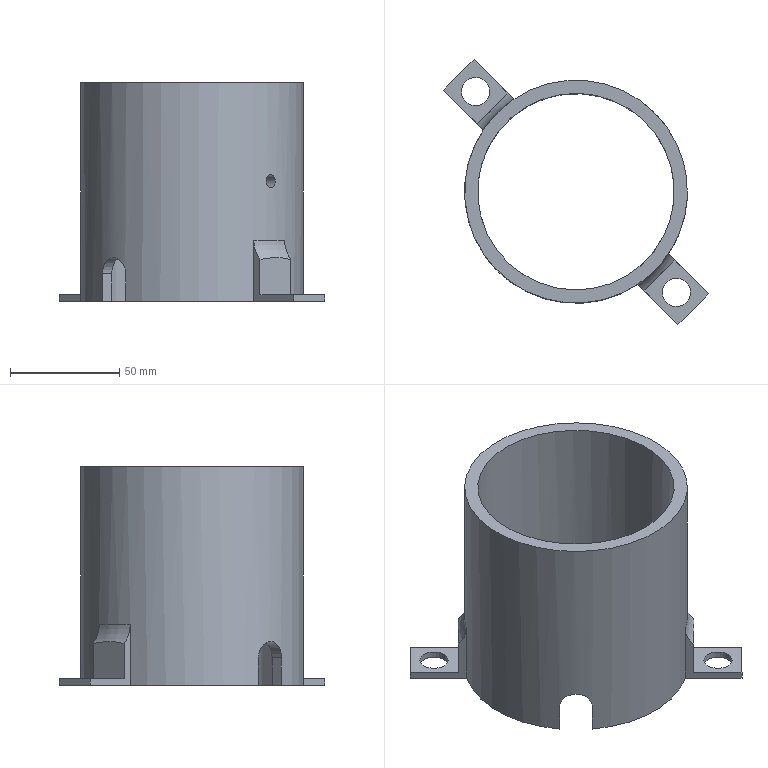Part | NX | features solid 2 | 1 solid | 26 faces | box 121.622 x 121.622 x 100 mm | volume 182276 mm3 | plane 17 | cylinder 7 | torus 2 | commonest cylinder face diameters 13 x2 15 x2 6 x1 90 x1 102 x1
STEP:
#1=CARTESIAN_POINT('',(1436.366,353.634,10.));
#2=VERTEX_POINT('',#1);
#3=CARTESIAN_POINT('',(1440.962,349.038,10.));
#4=DIRECTION('',(0.,0.,-1.));
#5=DIRECTION('',(-0.7071,0.7071,0.));
#6=AXIS2_PLACEMENT_3D('',#3,#4,#5);
#7=CIRCLE('',#6,6.5);
#8=EDGE_CURVE('',#2,#2,#7,.T.);
#9=ORIENTED_EDGE('',*,*,#8,.F.);
#10=EDGE_LOOP('',(#9));
#11=FACE_BOUND('',#10,.T.);
#12=CARTESIAN_POINT('',(1435.974,425.367,10.));
#13=VERTEX_POINT('',#12);
#14=CARTESIAN_POINT('',(1437.433,366.709,10.));
#15=VERTEX_POINT('',#14);
#16=CARTESIAN_POINT('',(1395.,395.,10.));
#17=DIRECTION('',(0.,0.,-1.));
#18=DIRECTION('',(-0.9659,-0.2588,0.));
#19=AXIS2_PLACEMENT_3D('',#16,#17,#18);
#20=CIRCLE('',#19,51.);
#21=EDGE_CURVE('',#13,#15,#20,.T.);
#22=ORIENTED_EDGE('',*,*,#21,.T.);
#23=CARTESIAN_POINT('',(1455.811,348.331,10.));
#24=VERTEX_POINT('',#23);
#25=CARTESIAN_POINT('',(1440.255,363.887,10.));
#26=DIRECTION('',(0.7071,-0.7071,0.));
#27=VECTOR('',#26,1000.);
#28=LINE('',#25,#27);
#29=EDGE_CURVE('',#15,#24,#28,.T.);
#30=ORIENTED_EDGE('',*,*,#29,.T.);
#31=CARTESIAN_POINT('',(1441.669,334.189,10.));
#32=VERTEX_POINT('',#31);
#33=CARTESIAN_POINT('',(1441.669,334.189,10.));
#34=DIRECTION('',(0.7071,0.7071,0.));
#35=VECTOR('',#34,1000.);
#36=LINE('',#33,#35);
#37=EDGE_CURVE('',#32,#24,#36,.T.);
#38=ORIENTED_EDGE('',*,*,#37,.F.);
#39=CARTESIAN_POINT('',(1423.291,352.567,10.));
#40=VERTEX_POINT('',#39);
#41=CARTESIAN_POINT('',(1432.477,343.381,10.));
#42=DIRECTION('',(-0.7071,0.7071,0.));
#43=VECTOR('',#42,1000.);
#44=LINE('',#41,#43);
#45=EDGE_CURVE('',#32,#40,#44,.T.);
#46=ORIENTED_EDGE('',*,*,#45,.T.);
#47=CARTESIAN_POINT('',(1364.633,354.026,10.));
#48=VERTEX_POINT('',#47);
#49=CARTESIAN_POINT('',(1395.,395.,10.));
#50=DIRECTION('',(0.,0.,-1.));
#51=DIRECTION('',(-0.9659,-0.2588,0.));
#52=AXIS2_PLACEMENT_3D('',#49,#50,#51);
#53=CIRCLE('',#52,51.);
#54=EDGE_CURVE('',#40,#48,#53,.T.);
#55=ORIENTED_EDGE('',*,*,#54,.T.);
#56=CARTESIAN_POINT('',(1368.929,358.322,10.));
#57=VERTEX_POINT('',#56);
#58=CARTESIAN_POINT('',(1400.303,389.697,10.));
#59=DIRECTION('',(-0.7071,-0.7071,0.));
#60=VECTOR('',#59,1000.);
#61=LINE('',#58,#60);
#62=EDGE_CURVE('',#57,#48,#61,.T.);
#63=ORIENTED_EDGE('',*,*,#62,.F.);
#64=CARTESIAN_POINT('',(1431.678,421.071,10.));
#65=VERTEX_POINT('',#64);
#66=CARTESIAN_POINT('',(1395.,395.,10.));
#67=DIRECTION('',(0.,0.,-1.));
#68=DIRECTION('',(-0.9659,-0.2588,0.));
#69=AXIS2_PLACEMENT_3D('',#66,#67,#68);
#70=CIRCLE('',#69,45.);
#71=EDGE_CURVE('',#65,#57,#70,.T.);
#72=ORIENTED_EDGE('',*,*,#71,.F.);
#73=CARTESIAN_POINT('',(1400.303,389.697,10.));
#74=DIRECTION('',(-0.7071,-0.7071,0.));
#75=VECTOR('',#74,1000.);
#76=LINE('',#73,#75);
#77=EDGE_CURVE('',#13,#65,#76,.T.);
#78=ORIENTED_EDGE('',*,*,#77,.F.);
#79=EDGE_LOOP('',(#22,#30,#38,#46,#55,#63,#72,#78));
#80=FACE_BOUND('',#79,.T.);
#81=CARTESIAN_POINT('',(1395.,395.,10.));
#82=DIRECTION('',(0.,0.,1.));
#83=DIRECTION('',(-0.7071,0.7071,0.));
#84=AXIS2_PLACEMENT_3D('',#81,#82,#83);
#85=PLANE('',#84);
#86=ADVANCED_FACE('',(#11,#80),#85,.F.);
#87=CARTESIAN_POINT('',(1430.87,358.746,62.012));
#88=VERTEX_POINT('',#87);
#89=CARTESIAN_POINT('',(1429.215,357.17,62.873));
#90=CARTESIAN_POINT('',(1430.865,358.71,61.688));
#91=CARTESIAN_POINT('',(1432.545,360.466,62.447));
#92=CARTESIAN_POINT('',(1433.326,361.356,64.697));
#93=CARTESIAN_POINT('',(1432.83,360.784,67.128));
#94=CARTESIAN_POINT('',(1431.29,359.136,68.311));
#95=CARTESIAN_POINT('',(1429.537,357.457,67.556));
#96=CARTESIAN_POINT('',(1428.644,356.674,65.304));
#97=CARTESIAN_POINT('',(1429.215,357.17,62.873));
#98=CARTESIAN_POINT('',(1430.865,358.71,61.688));
#99=CARTESIAN_POINT('',(1432.545,360.466,62.447));
#100=B_SPLINE_CURVE_WITH_KNOTS('',3,(#89,#90,#91,#92,#93,#94,#95,#96,#97,#98,#99),.UNSPECIFIED.,.T.,.F.,(1,1,1,1,1,1,1,1,1,1,1,1,1,1,1),(-0.007035,-0.00469,-0.002345,0.,0.002345,0.00469,0.007035,0.00938,0.01173,0.01407,0.01642,0.01876,0.02111,0.02345,0.0258),.UNSPECIFIED.);
#101=EDGE_CURVE('',#88,#88,#100,.T.);
#102=ORIENTED_EDGE('',*,*,#101,.F.);
#103=EDGE_LOOP('',(#102));
#104=FACE_BOUND('',#103,.T.);
#105=CARTESIAN_POINT('',(1444.262,408.2,110.));
#106=VERTEX_POINT('',#105);
#107=CARTESIAN_POINT('',(1395.,395.,110.));
#108=DIRECTION('',(0.,0.,-1.));
#109=DIRECTION('',(0.9659,0.2588,0.));
#110=AXIS2_PLACEMENT_3D('',#107,#108,#109);
#111=CIRCLE('',#110,51.);
#112=EDGE_CURVE('',#106,#106,#111,.T.);
#113=ORIENTED_EDGE('',*,*,#112,.T.);
#114=EDGE_LOOP('',(#113));
#115=FACE_BOUND('',#114,.T.);
#116=CARTESIAN_POINT('',(1425.367,435.974,22.5));
#117=VERTEX_POINT('',#116);
#118=CARTESIAN_POINT('',(1435.974,425.367,22.5));
#119=VERTEX_POINT('',#118);
#120=CARTESIAN_POINT('',(1425.367,435.974,22.5));
#121=CARTESIAN_POINT('',(1425.367,435.974,24.46));
#122=CARTESIAN_POINT('',(1426.705,435.029,28.37));
#123=CARTESIAN_POINT('',(1431.168,431.152,30.816));
#124=CARTESIAN_POINT('',(1435.022,426.713,28.365));
#125=CARTESIAN_POINT('',(1435.974,425.367,24.48));
#126=CARTESIAN_POINT('',(1435.974,425.367,22.5));
#127=B_SPLINE_CURVE_WITH_KNOTS('',3,(#120,#121,#122,#123,#124,#125,#126),.UNSPECIFIED.,.F.,.F.,(4,1,1,1,4),(0.03594,0.04181,0.04768,0.05355,0.05942),.UNSPECIFIED.);
#128=EDGE_CURVE('',#117,#119,#127,.T.);
#129=ORIENTED_EDGE('',*,*,#128,.F.);
#130=CARTESIAN_POINT('',(1425.367,435.974,10.));
#131=VERTEX_POINT('',#130);
#132=CARTESIAN_POINT('',(1425.367,435.974,120.));
#133=DIRECTION('',(0.,0.,-1.));
#134=VECTOR('',#133,1000.);
#135=LINE('',#132,#134);
#136=EDGE_CURVE('',#131,#117,#135,.F.);
#137=ORIENTED_EDGE('',*,*,#136,.F.);
#138=CARTESIAN_POINT('',(1366.709,437.433,10.));
#139=VERTEX_POINT('',#138);
#140=CARTESIAN_POINT('',(1395.,395.,10.));
#141=DIRECTION('',(0.,0.,-1.));
#142=DIRECTION('',(-0.9659,-0.2588,0.));
#143=AXIS2_PLACEMENT_3D('',#140,#141,#142);
#144=CIRCLE('',#143,51.);
#145=EDGE_CURVE('',#139,#131,#144,.T.);
#146=ORIENTED_EDGE('',*,*,#145,.F.);
#147=CARTESIAN_POINT('',(1366.709,437.433,38.));
#148=VERTEX_POINT('',#147);
#149=CARTESIAN_POINT('',(1366.709,437.433,10.));
#150=DIRECTION('',(0.,0.,-1.));
#151=VECTOR('',#150,1000.);
#152=LINE('',#149,#151);
#153=EDGE_CURVE('',#139,#148,#152,.F.);
#154=ORIENTED_EDGE('',*,*,#153,.T.);
#155=CARTESIAN_POINT('',(1352.567,423.291,38.));
#156=VERTEX_POINT('',#155);
#157=CARTESIAN_POINT('',(1395.,395.,38.));
#158=DIRECTION('',(0.,0.,1.));
#159=DIRECTION('',(0.9659,0.2588,0.));
#160=AXIS2_PLACEMENT_3D('',#157,#158,#159);
#161=CIRCLE('',#160,51.);
#162=EDGE_CURVE('',#156,#148,#161,.F.);
#163=ORIENTED_EDGE('',*,*,#162,.F.);
#164=CARTESIAN_POINT('',(1352.567,423.291,10.));
#165=VERTEX_POINT('',#164);
#166=CARTESIAN_POINT('',(1352.567,423.291,120.));
#167=DIRECTION('',(0.,0.,-1.));
#168=VECTOR('',#167,1000.);
#169=LINE('',#166,#168);
#170=EDGE_CURVE('',#156,#165,#169,.T.);
#171=ORIENTED_EDGE('',*,*,#170,.T.);
#172=CARTESIAN_POINT('',(1354.026,364.633,10.));
#173=VERTEX_POINT('',#172);
#174=CARTESIAN_POINT('',(1395.,395.,10.));
#175=DIRECTION('',(0.,0.,-1.));
#176=DIRECTION('',(-0.9659,-0.2588,0.));
#177=AXIS2_PLACEMENT_3D('',#174,#175,#176);
#178=CIRCLE('',#177,51.);
#179=EDGE_CURVE('',#173,#165,#178,.T.);
#180=ORIENTED_EDGE('',*,*,#179,.F.);
#181=CARTESIAN_POINT('',(1354.026,364.633,22.5));
#182=VERTEX_POINT('',#181);
#183=CARTESIAN_POINT('',(1354.026,364.633,120.));
#184=DIRECTION('',(0.,0.,-1.));
#185=VECTOR('',#184,1000.);
#186=LINE('',#183,#185);
#187=EDGE_CURVE('',#182,#173,#186,.T.);
#188=ORIENTED_EDGE('',*,*,#187,.F.);
#189=CARTESIAN_POINT('',(1364.633,354.026,22.5));
#190=VERTEX_POINT('',#189);
#191=CARTESIAN_POINT('',(1364.633,354.026,22.5));
#192=CARTESIAN_POINT('',(1364.633,354.026,24.483));
#193=CARTESIAN_POINT('',(1363.29,354.975,28.366));
#194=CARTESIAN_POINT('',(1358.835,358.845,30.816));
#195=CARTESIAN_POINT('',(1354.974,363.292,28.369));
#196=CARTESIAN_POINT('',(1354.026,364.633,24.459));
#197=CARTESIAN_POINT('',(1354.026,364.633,22.5));
#198=B_SPLINE_CURVE_WITH_KNOTS('',3,(#191,#192,#193,#194,#195,#196,#197),.UNSPECIFIED.,.F.,.F.,(4,1,1,1,4),(0.03522,0.04109,0.04696,0.05283,0.0587),.UNSPECIFIED.);
#199=EDGE_CURVE('',#190,#182,#198,.T.);
#200=ORIENTED_EDGE('',*,*,#199,.F.);
#201=CARTESIAN_POINT('',(1364.633,354.026,120.));
#202=DIRECTION('',(0.,0.,-1.));
#203=VECTOR('',#202,1000.);
#204=LINE('',#201,#203);
#205=EDGE_CURVE('',#48,#190,#204,.F.);
#206=ORIENTED_EDGE('',*,*,#205,.F.);
#207=ORIENTED_EDGE('',*,*,#54,.F.);
#208=CARTESIAN_POINT('',(1423.291,352.567,38.));
#209=VERTEX_POINT('',#208);
#210=CARTESIAN_POINT('',(1423.291,352.567,10.));
#211=DIRECTION('',(0.,0.,-1.));
#212=VECTOR('',#211,1000.);
#213=LINE('',#210,#212);
#214=EDGE_CURVE('',#40,#209,#213,.F.);
#215=ORIENTED_EDGE('',*,*,#214,.T.);
#216=CARTESIAN_POINT('',(1437.433,366.709,38.));
#217=VERTEX_POINT('',#216);
#218=CARTESIAN_POINT('',(1395.,395.,38.));
#219=DIRECTION('',(0.,0.,1.));
#220=DIRECTION('',(0.9659,0.2588,0.));
#221=AXIS2_PLACEMENT_3D('',#218,#219,#220);
#222=CIRCLE('',#221,51.);
#223=EDGE_CURVE('',#217,#209,#222,.F.);
#224=ORIENTED_EDGE('',*,*,#223,.F.);
#225=CARTESIAN_POINT('',(1437.433,366.709,120.));
#226=DIRECTION('',(0.,0.,-1.));
#227=VECTOR('',#226,1000.);
#228=LINE('',#225,#227);
#229=EDGE_CURVE('',#217,#15,#228,.T.);
#230=ORIENTED_EDGE('',*,*,#229,.T.);
#231=ORIENTED_EDGE('',*,*,#21,.F.);
#232=CARTESIAN_POINT('',(1435.974,425.367,120.));
#233=DIRECTION('',(0.,0.,-1.));
#234=VECTOR('',#233,1000.);
#235=LINE('',#232,#234);
#236=EDGE_CURVE('',#119,#13,#235,.T.);
#237=ORIENTED_EDGE('',*,*,#236,.F.);
#238=EDGE_LOOP('',(#129,#137,#146,#154,#163,#171,#180,#188,#200,#206,#207,#215,#224,#230,#231,#237));
#239=FACE_BOUND('',#238,.T.);
#240=CARTESIAN_POINT('',(1395.,395.,120.));
#241=DIRECTION('',(0.,0.,-1.));
#242=DIRECTION('',(0.7071,-0.7071,0.));
#243=AXIS2_PLACEMENT_3D('',#240,#241,#242);
#244=CYLINDRICAL_SURFACE('',#243,51.);
#245=ADVANCED_FACE('',(#104,#115,#239),#244,.T.);
#246=CARTESIAN_POINT('',(1431.678,421.071,22.5));
#247=VERTEX_POINT('',#246);
#248=CARTESIAN_POINT('',(1431.678,421.071,120.));
#249=DIRECTION('',(0.,0.,-1.));
#250=VECTOR('',#249,1000.);
#251=LINE('',#248,#250);
#252=EDGE_CURVE('',#247,#65,#251,.T.);
#253=ORIENTED_EDGE('',*,*,#252,.T.);
#254=ORIENTED_EDGE('',*,*,#71,.T.);
#255=CARTESIAN_POINT('',(1368.929,358.322,22.5));
#256=VERTEX_POINT('',#255);
#257=CARTESIAN_POINT('',(1368.929,358.322,120.));
#258=DIRECTION('',(0.,0.,-1.));
#259=VECTOR('',#258,1000.);
#260=LINE('',#257,#259);
#261=EDGE_CURVE('',#57,#256,#260,.F.);
#262=ORIENTED_EDGE('',*,*,#261,.T.);
#263=CARTESIAN_POINT('',(1358.322,368.929,22.5));
#264=VERTEX_POINT('',#263);
#265=CARTESIAN_POINT('',(1368.929,358.322,22.5));
#266=CARTESIAN_POINT('',(1368.929,358.322,24.482));
#267=CARTESIAN_POINT('',(1367.559,359.244,28.366));
#268=CARTESIAN_POINT('',(1363.064,363.075,30.817));
#269=CARTESIAN_POINT('',(1359.243,367.561,28.368));
#270=CARTESIAN_POINT('',(1358.322,368.929,24.46));
#271=CARTESIAN_POINT('',(1358.322,368.929,22.5));
#272=B_SPLINE_CURVE_WITH_KNOTS('',3,(#265,#266,#267,#268,#269,#270,#271),.UNSPECIFIED.,.F.,.F.,(4,1,1,1,4),(0.03524,0.04111,0.04698,0.05285,0.05872),.UNSPECIFIED.);
#273=EDGE_CURVE('',#256,#264,#272,.T.);
#274=ORIENTED_EDGE('',*,*,#273,.T.);
#275=CARTESIAN_POINT('',(1358.322,368.929,10.));
#276=VERTEX_POINT('',#275);
#277=CARTESIAN_POINT('',(1358.322,368.929,120.));
#278=DIRECTION('',(0.,0.,-1.));
#279=VECTOR('',#278,1000.);
#280=LINE('',#277,#279);
#281=EDGE_CURVE('',#264,#276,#280,.T.);
#282=ORIENTED_EDGE('',*,*,#281,.T.);
#283=CARTESIAN_POINT('',(1421.071,431.678,10.));
#284=VERTEX_POINT('',#283);
#285=CARTESIAN_POINT('',(1395.,395.,10.));
#286=DIRECTION('',(0.,0.,-1.));
#287=DIRECTION('',(-0.9659,-0.2588,0.));
#288=AXIS2_PLACEMENT_3D('',#285,#286,#287);
#289=CIRCLE('',#288,45.);
#290=EDGE_CURVE('',#276,#284,#289,.T.);
#291=ORIENTED_EDGE('',*,*,#290,.T.);
#292=CARTESIAN_POINT('',(1421.071,431.678,22.5));
#293=VERTEX_POINT('',#292);
#294=CARTESIAN_POINT('',(1421.071,431.678,120.));
#295=DIRECTION('',(0.,0.,-1.));
#296=VECTOR('',#295,1000.);
#297=LINE('',#294,#296);
#298=EDGE_CURVE('',#284,#293,#297,.F.);
#299=ORIENTED_EDGE('',*,*,#298,.T.);
#300=CARTESIAN_POINT('',(1421.071,431.678,22.5));
#301=CARTESIAN_POINT('',(1421.071,431.678,24.485));
#302=CARTESIAN_POINT('',(1422.445,430.753,28.364));
#303=CARTESIAN_POINT('',(1426.924,426.936,30.816));
#304=CARTESIAN_POINT('',(1430.753,422.446,28.37));
#305=CARTESIAN_POINT('',(1431.678,421.071,24.485));
#306=CARTESIAN_POINT('',(1431.678,421.071,22.5));
#307=B_SPLINE_CURVE_WITH_KNOTS('',3,(#300,#301,#302,#303,#304,#305,#306),.UNSPECIFIED.,.F.,.F.,(4,1,1,1,4),(0.,0.005871,0.01174,0.01761,0.02348),.UNSPECIFIED.);
#308=EDGE_CURVE('',#293,#247,#307,.T.);
#309=ORIENTED_EDGE('',*,*,#308,.T.);
#310=EDGE_LOOP('',(#253,#254,#262,#274,#282,#291,#299,#309));
#311=FACE_BOUND('',#310,.T.);
#312=CARTESIAN_POINT('',(1426.631,362.992,62.012));
#313=VERTEX_POINT('',#312);
#314=CARTESIAN_POINT('',(1424.97,361.42,62.869));
#315=CARTESIAN_POINT('',(1426.628,362.955,61.688));
#316=CARTESIAN_POINT('',(1428.302,364.714,62.451));
#317=CARTESIAN_POINT('',(1429.073,365.609,64.702));
#318=CARTESIAN_POINT('',(1428.579,365.029,67.132));
#319=CARTESIAN_POINT('',(1427.046,363.373,68.311));
#320=CARTESIAN_POINT('',(1425.288,361.7,67.552));
#321=CARTESIAN_POINT('',(1424.391,360.926,65.299));
#322=CARTESIAN_POINT('',(1424.97,361.42,62.869));
#323=CARTESIAN_POINT('',(1426.628,362.955,61.688));
#324=CARTESIAN_POINT('',(1428.302,364.714,62.451));
#325=B_SPLINE_CURVE_WITH_KNOTS('',3,(#314,#315,#316,#317,#318,#319,#320,#321,#322,#323,#324),.UNSPECIFIED.,.T.,.F.,(1,1,1,1,1,1,1,1,1,1,1,1,1,1,1),(-0.007036,-0.00469,-0.002345,0.,0.002345,0.00469,0.007036,0.009381,0.01173,0.01407,0.01642,0.01876,0.02111,0.02345,0.0258),.UNSPECIFIED.);
#326=EDGE_CURVE('',#313,#313,#325,.T.);
#327=ORIENTED_EDGE('',*,*,#326,.T.);
#328=EDGE_LOOP('',(#327));
#329=FACE_BOUND('',#328,.T.);
#330=CARTESIAN_POINT('',(1438.467,406.647,110.));
#331=VERTEX_POINT('',#330);
#332=CARTESIAN_POINT('',(1395.,395.,110.));
#333=DIRECTION('',(0.,0.,-1.));
#334=DIRECTION('',(0.9659,0.2588,0.));
#335=AXIS2_PLACEMENT_3D('',#332,#333,#334);
#336=CIRCLE('',#335,45.);
#337=EDGE_CURVE('',#331,#331,#336,.T.);
#338=ORIENTED_EDGE('',*,*,#337,.F.);
#339=EDGE_LOOP('',(#338));
#340=FACE_BOUND('',#339,.T.);
#341=CARTESIAN_POINT('',(1395.,395.,120.));
#342=DIRECTION('',(0.,0.,-1.));
#343=DIRECTION('',(0.7071,-0.7071,0.));
#344=AXIS2_PLACEMENT_3D('',#341,#342,#343);
#345=CYLINDRICAL_SURFACE('',#344,45.);
#346=ADVANCED_FACE('',(#311,#329,#340),#345,.F.);
#347=ORIENTED_EDGE('',*,*,#337,.T.);
#348=EDGE_LOOP('',(#347));
#349=FACE_BOUND('',#348,.T.);
#350=ORIENTED_EDGE('',*,*,#112,.F.);
#351=EDGE_LOOP('',(#350));
#352=FACE_BOUND('',#351,.T.);
#353=CARTESIAN_POINT('',(1395.,395.,110.));
#354=DIRECTION('',(0.,0.,1.));
#355=DIRECTION('',(-0.7071,0.7071,0.));
#356=AXIS2_PLACEMENT_3D('',#353,#354,#355);
#357=PLANE('',#356);
#358=ADVANCED_FACE('',(#349,#352),#357,.T.);
#359=ORIENTED_EDGE('',*,*,#290,.F.);
#360=CARTESIAN_POINT('',(1389.697,400.303,10.));
#361=DIRECTION('',(0.7071,0.7071,0.));
#362=VECTOR('',#361,1000.);
#363=LINE('',#360,#362);
#364=EDGE_CURVE('',#173,#276,#363,.T.);
#365=ORIENTED_EDGE('',*,*,#364,.F.);
#366=ORIENTED_EDGE('',*,*,#179,.T.);
#367=CARTESIAN_POINT('',(1334.189,441.669,10.));
#368=VERTEX_POINT('',#367);
#369=CARTESIAN_POINT('',(1349.745,426.113,10.));
#370=DIRECTION('',(-0.7071,0.7071,0.));
#371=VECTOR('',#370,1000.);
#372=LINE('',#369,#371);
#373=EDGE_CURVE('',#165,#368,#372,.T.);
#374=ORIENTED_EDGE('',*,*,#373,.T.);
#375=CARTESIAN_POINT('',(1348.331,455.811,10.));
#376=VERTEX_POINT('',#375);
#377=CARTESIAN_POINT('',(1348.331,455.811,10.));
#378=DIRECTION('',(-0.7071,-0.7071,0.));
#379=VECTOR('',#378,1000.);
#380=LINE('',#377,#379);
#381=EDGE_CURVE('',#376,#368,#380,.T.);
#382=ORIENTED_EDGE('',*,*,#381,.F.);
#383=CARTESIAN_POINT('',(1357.523,446.619,10.));
#384=DIRECTION('',(0.7071,-0.7071,0.));
#385=VECTOR('',#384,1000.);
#386=LINE('',#383,#385);
#387=EDGE_CURVE('',#376,#139,#386,.T.);
#388=ORIENTED_EDGE('',*,*,#387,.T.);
#389=ORIENTED_EDGE('',*,*,#145,.T.);
#390=CARTESIAN_POINT('',(1389.697,400.303,10.));
#391=DIRECTION('',(0.7071,0.7071,0.));
#392=VECTOR('',#391,1000.);
#393=LINE('',#390,#392);
#394=EDGE_CURVE('',#284,#131,#393,.T.);
#395=ORIENTED_EDGE('',*,*,#394,.F.);
#396=EDGE_LOOP('',(#359,#365,#366,#374,#382,#388,#389,#395));
#397=FACE_BOUND('',#396,.T.);
#398=CARTESIAN_POINT('',(1344.442,445.558,10.));
#399=VERTEX_POINT('',#398);
#400=CARTESIAN_POINT('',(1349.038,440.962,10.));
#401=DIRECTION('',(0.,0.,-1.));
#402=DIRECTION('',(-0.7071,0.7071,0.));
#403=AXIS2_PLACEMENT_3D('',#400,#401,#402);
#404=CIRCLE('',#403,6.5);
#405=EDGE_CURVE('',#399,#399,#404,.T.);
#406=ORIENTED_EDGE('',*,*,#405,.F.);
#407=EDGE_LOOP('',(#406));
#408=FACE_BOUND('',#407,.T.);
#409=CARTESIAN_POINT('',(1395.,395.,10.));
#410=DIRECTION('',(0.,0.,1.));
#411=DIRECTION('',(-0.7071,0.7071,0.));
#412=AXIS2_PLACEMENT_3D('',#409,#410,#411);
#413=PLANE('',#412);
#414=ADVANCED_FACE('',(#397,#408),#413,.F.);
#415=ORIENTED_EDGE('',*,*,#45,.F.);
#416=CARTESIAN_POINT('',(1441.669,334.189,13.));
#417=VERTEX_POINT('',#416);
#418=CARTESIAN_POINT('',(1441.669,334.189,13.));
#419=DIRECTION('',(0.,0.,-1.));
#420=VECTOR('',#419,1000.);
#421=LINE('',#418,#420);
#422=EDGE_CURVE('',#417,#32,#421,.T.);
#423=ORIENTED_EDGE('',*,*,#422,.F.);
#424=CARTESIAN_POINT('',(1426.113,349.745,13.));
#425=VERTEX_POINT('',#424);
#426=CARTESIAN_POINT('',(1432.477,343.381,13.));
#427=DIRECTION('',(0.7071,-0.7071,0.));
#428=VECTOR('',#427,1000.);
#429=LINE('',#426,#428);
#430=EDGE_CURVE('',#425,#417,#429,.T.);
#431=ORIENTED_EDGE('',*,*,#430,.F.);
#432=CARTESIAN_POINT('',(1426.113,349.745,29.13));
#433=VERTEX_POINT('',#432);
#434=CARTESIAN_POINT('',(1426.113,349.745,35.));
#435=DIRECTION('',(0.,0.,-1.));
#436=VECTOR('',#435,1000.);
#437=LINE('',#434,#436);
#438=EDGE_CURVE('',#433,#425,#437,.T.);
#439=ORIENTED_EDGE('',*,*,#438,.F.);
#440=CARTESIAN_POINT('',(1423.291,352.567,38.));
#441=CARTESIAN_POINT('',(1423.291,352.567,34.628));
#442=CARTESIAN_POINT('',(1424.362,351.496,31.348));
#443=CARTESIAN_POINT('',(1426.113,349.745,29.13));
#444=B_SPLINE_CURVE_WITH_KNOTS('',3,(#440,#441,#442,#443),.UNSPECIFIED.,.F.,.F.,(4,4),(0.,0.00997),.UNSPECIFIED.);
#445=EDGE_CURVE('',#209,#433,#444,.T.);
#446=ORIENTED_EDGE('',*,*,#445,.F.);
#447=ORIENTED_EDGE('',*,*,#214,.F.);
#448=EDGE_LOOP('',(#415,#423,#431,#439,#446,#447));
#449=FACE_BOUND('',#448,.T.);
#450=CARTESIAN_POINT('',(1432.477,343.381,35.));
#451=DIRECTION('',(0.7071,0.7071,0.));
#452=DIRECTION('',(0.7071,-0.7071,0.));
#453=AXIS2_PLACEMENT_3D('',#450,#451,#452);
#454=PLANE('',#453);
#455=ADVANCED_FACE('',(#449),#454,.F.);
#456=CARTESIAN_POINT('',(1440.255,363.887,29.13));
#457=VERTEX_POINT('',#456);
#458=CARTESIAN_POINT('',(1440.255,363.887,13.));
#459=VERTEX_POINT('',#458);
#460=CARTESIAN_POINT('',(1440.255,363.887,35.));
#461=DIRECTION('',(0.,0.,-1.));
#462=VECTOR('',#461,1000.);
#463=LINE('',#460,#462);
#464=EDGE_CURVE('',#457,#459,#463,.T.);
#465=ORIENTED_EDGE('',*,*,#464,.T.);
#466=CARTESIAN_POINT('',(1455.811,348.331,13.));
#467=VERTEX_POINT('',#466);
#468=CARTESIAN_POINT('',(1462.175,341.967,13.));
#469=DIRECTION('',(-0.7071,0.7071,0.));
#470=VECTOR('',#469,1000.);
#471=LINE('',#468,#470);
#472=EDGE_CURVE('',#467,#459,#471,.T.);
#473=ORIENTED_EDGE('',*,*,#472,.F.);
#474=CARTESIAN_POINT('',(1455.811,348.331,13.));
#475=DIRECTION('',(0.,0.,-1.));
#476=VECTOR('',#475,1000.);
#477=LINE('',#474,#476);
#478=EDGE_CURVE('',#467,#24,#477,.T.);
#479=ORIENTED_EDGE('',*,*,#478,.T.);
#480=ORIENTED_EDGE('',*,*,#29,.F.);
#481=ORIENTED_EDGE('',*,*,#229,.F.);
#482=CARTESIAN_POINT('',(1440.255,363.887,29.13));
#483=CARTESIAN_POINT('',(1438.495,365.647,31.359));
#484=CARTESIAN_POINT('',(1437.433,366.709,34.631));
#485=CARTESIAN_POINT('',(1437.433,366.709,38.));
#486=B_SPLINE_CURVE_WITH_KNOTS('',3,(#482,#483,#484,#485),.UNSPECIFIED.,.F.,.F.,(4,4),(0.00893,0.01889),.UNSPECIFIED.);
#487=EDGE_CURVE('',#457,#217,#486,.T.);
#488=ORIENTED_EDGE('',*,*,#487,.F.);
#489=EDGE_LOOP('',(#465,#473,#479,#480,#481,#488));
#490=FACE_BOUND('',#489,.T.);
#491=CARTESIAN_POINT('',(1440.255,363.887,35.));
#492=DIRECTION('',(-0.7071,-0.7071,0.));
#493=DIRECTION('',(-0.7071,0.7071,0.));
#494=AXIS2_PLACEMENT_3D('',#491,#492,#493);
#495=PLANE('',#494);
#496=ADVANCED_FACE('',(#490),#495,.F.);
#497=ORIENTED_EDGE('',*,*,#464,.F.);
#498=CARTESIAN_POINT('',(1426.113,349.745,29.13));
#499=CARTESIAN_POINT('',(1428.44,352.072,29.676));
#500=CARTESIAN_POINT('',(1431.947,355.58,30.244));
#501=CARTESIAN_POINT('',(1436.083,359.715,29.934));
#502=CARTESIAN_POINT('',(1438.173,361.805,29.579));
#503=CARTESIAN_POINT('',(1439.351,362.984,29.337));
#504=CARTESIAN_POINT('',(1439.976,363.608,29.195));
#505=CARTESIAN_POINT('',(1440.255,363.887,29.13));
#506=B_SPLINE_CURVE_WITH_KNOTS('',3,(#498,#499,#500,#501,#502,#503,#504,#505),.UNSPECIFIED.,.F.,.F.,(4,1,1,1,1,4),(0.2077,0.2173,0.2221,0.2245,0.2257,0.2269),.UNSPECIFIED.);
#507=EDGE_CURVE('',#457,#433,#506,.F.);
#508=ORIENTED_EDGE('',*,*,#507,.T.);
#509=ORIENTED_EDGE('',*,*,#438,.T.);
#510=CARTESIAN_POINT('',(1440.255,363.887,13.));
#511=DIRECTION('',(-0.7071,-0.7071,0.));
#512=VECTOR('',#511,1000.);
#513=LINE('',#510,#512);
#514=EDGE_CURVE('',#459,#425,#513,.T.);
#515=ORIENTED_EDGE('',*,*,#514,.F.);
#516=EDGE_LOOP('',(#497,#508,#509,#515));
#517=FACE_BOUND('',#516,.T.);
#518=CARTESIAN_POINT('',(1440.255,363.887,35.));
#519=DIRECTION('',(-0.7071,0.7071,0.));
#520=DIRECTION('',(0.,0.,-1.));
#521=AXIS2_PLACEMENT_3D('',#518,#519,#520);
#522=PLANE('',#521);
#523=ADVANCED_FACE('',(#517),#522,.F.);
#524=ORIENTED_EDGE('',*,*,#387,.F.);
#525=CARTESIAN_POINT('',(1348.331,455.811,13.));
#526=VERTEX_POINT('',#525);
#527=CARTESIAN_POINT('',(1348.331,455.811,13.));
#528=DIRECTION('',(0.,0.,-1.));
#529=VECTOR('',#528,1000.);
#530=LINE('',#527,#529);
#531=EDGE_CURVE('',#526,#376,#530,.T.);
#532=ORIENTED_EDGE('',*,*,#531,.F.);
#533=CARTESIAN_POINT('',(1363.887,440.255,13.));
#534=VERTEX_POINT('',#533);
#535=CARTESIAN_POINT('',(1357.523,446.619,13.));
#536=DIRECTION('',(-0.7071,0.7071,0.));
#537=VECTOR('',#536,1000.);
#538=LINE('',#535,#537);
#539=EDGE_CURVE('',#534,#526,#538,.T.);
#540=ORIENTED_EDGE('',*,*,#539,.F.);
#541=CARTESIAN_POINT('',(1363.887,440.255,29.13));
#542=VERTEX_POINT('',#541);
#543=CARTESIAN_POINT('',(1363.887,440.255,35.));
#544=DIRECTION('',(0.,0.,-1.));
#545=VECTOR('',#544,1000.);
#546=LINE('',#543,#545);
#547=EDGE_CURVE('',#542,#534,#546,.T.);
#548=ORIENTED_EDGE('',*,*,#547,.F.);
#549=CARTESIAN_POINT('',(1366.709,437.433,38.));
#550=CARTESIAN_POINT('',(1366.709,437.433,34.628));
#551=CARTESIAN_POINT('',(1365.638,438.504,31.348));
#552=CARTESIAN_POINT('',(1363.887,440.255,29.13));
#553=B_SPLINE_CURVE_WITH_KNOTS('',3,(#549,#550,#551,#552),.UNSPECIFIED.,.F.,.F.,(4,4),(0.,0.00997),.UNSPECIFIED.);
#554=EDGE_CURVE('',#148,#542,#553,.T.);
#555=ORIENTED_EDGE('',*,*,#554,.F.);
#556=ORIENTED_EDGE('',*,*,#153,.F.);
#557=EDGE_LOOP('',(#524,#532,#540,#548,#555,#556));
#558=FACE_BOUND('',#557,.T.);
#559=CARTESIAN_POINT('',(1357.523,446.619,35.));
#560=DIRECTION('',(-0.7071,-0.7071,0.));
#561=DIRECTION('',(-0.7071,0.7071,0.));
#562=AXIS2_PLACEMENT_3D('',#559,#560,#561);
#563=PLANE('',#562);
#564=ADVANCED_FACE('',(#558),#563,.F.);
#565=CARTESIAN_POINT('',(1349.745,426.113,29.13));
#566=VERTEX_POINT('',#565);
#567=CARTESIAN_POINT('',(1349.745,426.113,13.));
#568=VERTEX_POINT('',#567);
#569=CARTESIAN_POINT('',(1349.745,426.113,35.));
#570=DIRECTION('',(0.,0.,-1.));
#571=VECTOR('',#570,1000.);
#572=LINE('',#569,#571);
#573=EDGE_CURVE('',#566,#568,#572,.T.);
#574=ORIENTED_EDGE('',*,*,#573,.T.);
#575=CARTESIAN_POINT('',(1334.189,441.669,13.));
#576=VERTEX_POINT('',#575);
#577=CARTESIAN_POINT('',(1327.825,448.033,13.));
#578=DIRECTION('',(0.7071,-0.7071,0.));
#579=VECTOR('',#578,1000.);
#580=LINE('',#577,#579);
#581=EDGE_CURVE('',#576,#568,#580,.T.);
#582=ORIENTED_EDGE('',*,*,#581,.F.);
#583=CARTESIAN_POINT('',(1334.189,441.669,13.));
#584=DIRECTION('',(0.,0.,-1.));
#585=VECTOR('',#584,1000.);
#586=LINE('',#583,#585);
#587=EDGE_CURVE('',#576,#368,#586,.T.);
#588=ORIENTED_EDGE('',*,*,#587,.T.);
#589=ORIENTED_EDGE('',*,*,#373,.F.);
#590=ORIENTED_EDGE('',*,*,#170,.F.);
#591=CARTESIAN_POINT('',(1349.745,426.113,29.13));
#592=CARTESIAN_POINT('',(1351.505,424.353,31.359));
#593=CARTESIAN_POINT('',(1352.567,423.291,34.631));
#594=CARTESIAN_POINT('',(1352.567,423.291,38.));
#595=B_SPLINE_CURVE_WITH_KNOTS('',3,(#591,#592,#593,#594),.UNSPECIFIED.,.F.,.F.,(4,4),(0.00893,0.01889),.UNSPECIFIED.);
#596=EDGE_CURVE('',#566,#156,#595,.T.);
#597=ORIENTED_EDGE('',*,*,#596,.F.);
#598=EDGE_LOOP('',(#574,#582,#588,#589,#590,#597));
#599=FACE_BOUND('',#598,.T.);
#600=CARTESIAN_POINT('',(1349.745,426.113,35.));
#601=DIRECTION('',(0.7071,0.7071,0.));
#602=DIRECTION('',(0.,0.,1.));
#603=AXIS2_PLACEMENT_3D('',#600,#601,#602);
#604=PLANE('',#603);
#605=ADVANCED_FACE('',(#599),#604,.F.);
#606=ORIENTED_EDGE('',*,*,#573,.F.);
#607=CARTESIAN_POINT('',(1363.887,440.255,29.13));
#608=CARTESIAN_POINT('',(1361.56,437.928,29.676));
#609=CARTESIAN_POINT('',(1358.053,434.42,30.244));
#610=CARTESIAN_POINT('',(1353.917,430.285,29.934));
#611=CARTESIAN_POINT('',(1351.827,428.195,29.579));
#612=CARTESIAN_POINT('',(1350.649,427.016,29.337));
#613=CARTESIAN_POINT('',(1350.024,426.392,29.195));
#614=CARTESIAN_POINT('',(1349.745,426.113,29.13));
#615=B_SPLINE_CURVE_WITH_KNOTS('',3,(#607,#608,#609,#610,#611,#612,#613,#614),.UNSPECIFIED.,.F.,.F.,(4,1,1,1,1,4),(0.2077,0.2173,0.2221,0.2245,0.2257,0.2269),.UNSPECIFIED.);
#616=EDGE_CURVE('',#566,#542,#615,.F.);
#617=ORIENTED_EDGE('',*,*,#616,.T.);
#618=ORIENTED_EDGE('',*,*,#547,.T.);
#619=CARTESIAN_POINT('',(1349.745,426.113,13.));
#620=DIRECTION('',(0.7071,0.7071,0.));
#621=VECTOR('',#620,1000.);
#622=LINE('',#619,#621);
#623=EDGE_CURVE('',#568,#534,#622,.T.);
#624=ORIENTED_EDGE('',*,*,#623,.F.);
#625=EDGE_LOOP('',(#606,#617,#618,#624));
#626=FACE_BOUND('',#625,.T.);
#627=CARTESIAN_POINT('',(1349.745,426.113,35.));
#628=DIRECTION('',(0.7071,-0.7071,0.));
#629=DIRECTION('',(0.,0.,1.));
#630=AXIS2_PLACEMENT_3D('',#627,#628,#629);
#631=PLANE('',#630);
#632=ADVANCED_FACE('',(#626),#631,.F.);
#633=ORIENTED_EDGE('',*,*,#381,.T.);
#634=ORIENTED_EDGE('',*,*,#587,.F.);
#635=CARTESIAN_POINT('',(1348.331,455.811,13.));
#636=DIRECTION('',(-0.7071,-0.7071,0.));
#637=VECTOR('',#636,1000.);
#638=LINE('',#635,#637);
#639=EDGE_CURVE('',#526,#576,#638,.T.);
#640=ORIENTED_EDGE('',*,*,#639,.F.);
#641=ORIENTED_EDGE('',*,*,#531,.T.);
#642=EDGE_LOOP('',(#633,#634,#640,#641));
#643=FACE_BOUND('',#642,.T.);
#644=CARTESIAN_POINT('',(1348.331,455.811,13.));
#645=DIRECTION('',(-0.7071,0.7071,0.));
#646=DIRECTION('',(0.,0.,-1.));
#647=AXIS2_PLACEMENT_3D('',#644,#645,#646);
#648=PLANE('',#647);
#649=ADVANCED_FACE('',(#643),#648,.T.);
#650=CARTESIAN_POINT('',(1344.442,445.558,13.));
#651=VERTEX_POINT('',#650);
#652=CARTESIAN_POINT('',(1349.038,440.962,13.));
#653=DIRECTION('',(0.,0.,-1.));
#654=DIRECTION('',(-0.7071,0.7071,0.));
#655=AXIS2_PLACEMENT_3D('',#652,#653,#654);
#656=CIRCLE('',#655,6.5);
#657=EDGE_CURVE('',#651,#651,#656,.T.);
#658=ORIENTED_EDGE('',*,*,#657,.F.);
#659=EDGE_LOOP('',(#658));
#660=FACE_BOUND('',#659,.T.);
#661=ORIENTED_EDGE('',*,*,#405,.T.);
#662=EDGE_LOOP('',(#661));
#663=FACE_BOUND('',#662,.T.);
#664=CARTESIAN_POINT('',(1349.038,440.962,13.));
#665=DIRECTION('',(0.,0.,-1.));
#666=DIRECTION('',(0.7071,-0.7071,0.));
#667=AXIS2_PLACEMENT_3D('',#664,#665,#666);
#668=CYLINDRICAL_SURFACE('',#667,6.5);
#669=ADVANCED_FACE('',(#660,#663),#668,.F.);
#670=ORIENTED_EDGE('',*,*,#639,.T.);
#671=ORIENTED_EDGE('',*,*,#581,.T.);
#672=ORIENTED_EDGE('',*,*,#623,.T.);
#673=ORIENTED_EDGE('',*,*,#539,.T.);
#674=EDGE_LOOP('',(#670,#671,#672,#673));
#675=FACE_BOUND('',#674,.T.);
#676=ORIENTED_EDGE('',*,*,#657,.T.);
#677=EDGE_LOOP('',(#676));
#678=FACE_BOUND('',#677,.T.);
#679=CARTESIAN_POINT('',(1327.825,448.033,13.));
#680=DIRECTION('',(0.,0.,-1.));
#681=DIRECTION('',(0.7071,-0.7071,0.));
#682=AXIS2_PLACEMENT_3D('',#679,#680,#681);
#683=PLANE('',#682);
#684=ADVANCED_FACE('',(#675,#678),#683,.F.);
#685=ORIENTED_EDGE('',*,*,#37,.T.);
#686=ORIENTED_EDGE('',*,*,#478,.F.);
#687=CARTESIAN_POINT('',(1441.669,334.189,13.));
#688=DIRECTION('',(0.7071,0.7071,0.));
#689=VECTOR('',#688,1000.);
#690=LINE('',#687,#689);
#691=EDGE_CURVE('',#417,#467,#690,.T.);
#692=ORIENTED_EDGE('',*,*,#691,.F.);
#693=ORIENTED_EDGE('',*,*,#422,.T.);
#694=EDGE_LOOP('',(#685,#686,#692,#693));
#695=FACE_BOUND('',#694,.T.);
#696=CARTESIAN_POINT('',(1441.669,334.189,13.));
#697=DIRECTION('',(0.7071,-0.7071,0.));
#698=DIRECTION('',(0.,0.,1.));
#699=AXIS2_PLACEMENT_3D('',#696,#697,#698);
#700=PLANE('',#699);
#701=ADVANCED_FACE('',(#695),#700,.T.);
#702=CARTESIAN_POINT('',(1436.366,353.634,13.));
#703=VERTEX_POINT('',#702);
#704=CARTESIAN_POINT('',(1440.962,349.038,13.));
#705=DIRECTION('',(0.,0.,-1.));
#706=DIRECTION('',(-0.7071,0.7071,0.));
#707=AXIS2_PLACEMENT_3D('',#704,#705,#706);
#708=CIRCLE('',#707,6.5);
#709=EDGE_CURVE('',#703,#703,#708,.T.);
#710=ORIENTED_EDGE('',*,*,#709,.F.);
#711=EDGE_LOOP('',(#710));
#712=FACE_BOUND('',#711,.T.);
#713=ORIENTED_EDGE('',*,*,#8,.T.);
#714=EDGE_LOOP('',(#713));
#715=FACE_BOUND('',#714,.T.);
#716=CARTESIAN_POINT('',(1440.962,349.038,13.));
#717=DIRECTION('',(0.,0.,-1.));
#718=DIRECTION('',(0.7071,-0.7071,0.));
#719=AXIS2_PLACEMENT_3D('',#716,#717,#718);
#720=CYLINDRICAL_SURFACE('',#719,6.5);
#721=ADVANCED_FACE('',(#712,#715),#720,.F.);
#722=ORIENTED_EDGE('',*,*,#691,.T.);
#723=ORIENTED_EDGE('',*,*,#472,.T.);
#724=ORIENTED_EDGE('',*,*,#514,.T.);
#725=ORIENTED_EDGE('',*,*,#430,.T.);
#726=EDGE_LOOP('',(#722,#723,#724,#725));
#727=FACE_BOUND('',#726,.T.);
#728=ORIENTED_EDGE('',*,*,#709,.T.);
#729=EDGE_LOOP('',(#728));
#730=FACE_BOUND('',#729,.T.);
#731=CARTESIAN_POINT('',(1462.175,341.967,13.));
#732=DIRECTION('',(0.,0.,-1.));
#733=DIRECTION('',(0.7071,-0.7071,0.));
#734=AXIS2_PLACEMENT_3D('',#731,#732,#733);
#735=PLANE('',#734);
#736=ADVANCED_FACE('',(#727,#730),#735,.F.);
#737=ORIENTED_EDGE('',*,*,#487,.T.);
#738=ORIENTED_EDGE('',*,*,#223,.T.);
#739=ORIENTED_EDGE('',*,*,#445,.T.);
#740=ORIENTED_EDGE('',*,*,#507,.F.);
#741=EDGE_LOOP('',(#737,#738,#739,#740));
#742=FACE_BOUND('',#741,.T.);
#743=CARTESIAN_POINT('',(1395.,395.,38.));
#744=DIRECTION('',(0.,0.,1.));
#745=DIRECTION('',(-0.7071,0.7071,0.));
#746=AXIS2_PLACEMENT_3D('',#743,#744,#745);
#747=TOROIDAL_SURFACE('',#746,63.,12.);
#748=ADVANCED_FACE('',(#742),#747,.F.);
#749=ORIENTED_EDGE('',*,*,#596,.T.);
#750=ORIENTED_EDGE('',*,*,#162,.T.);
#751=ORIENTED_EDGE('',*,*,#554,.T.);
#752=ORIENTED_EDGE('',*,*,#616,.F.);
#753=EDGE_LOOP('',(#749,#750,#751,#752));
#754=FACE_BOUND('',#753,.T.);
#755=CARTESIAN_POINT('',(1395.,395.,38.));
#756=DIRECTION('',(0.,0.,1.));
#757=DIRECTION('',(-0.7071,0.7071,0.));
#758=AXIS2_PLACEMENT_3D('',#755,#756,#757);
#759=TOROIDAL_SURFACE('',#758,63.,12.);
#760=ADVANCED_FACE('',(#754),#759,.F.);
#761=ORIENTED_EDGE('',*,*,#326,.F.);
#762=EDGE_LOOP('',(#761));
#763=FACE_BOUND('',#762,.T.);
#764=ORIENTED_EDGE('',*,*,#101,.T.);
#765=EDGE_LOOP('',(#764));
#766=FACE_BOUND('',#765,.T.);
#767=CARTESIAN_POINT('',(1395.,395.,65.));
#768=DIRECTION('',(0.7071,-0.7071,0.));
#769=DIRECTION('',(0.,0.,1.));
#770=AXIS2_PLACEMENT_3D('',#767,#768,#769);
#771=CYLINDRICAL_SURFACE('',#770,3.);
#772=ADVANCED_FACE('',(#763,#766),#771,.F.);
#773=CARTESIAN_POINT('',(1400.303,389.697,22.5));
#774=DIRECTION('',(0.7071,0.7071,0.));
#775=VECTOR('',#774,1000.);
#776=LINE('',#773,#775);
#777=EDGE_CURVE('',#190,#256,#776,.T.);
#778=ORIENTED_EDGE('',*,*,#777,.F.);
#779=ORIENTED_EDGE('',*,*,#199,.T.);
#780=CARTESIAN_POINT('',(1389.697,400.303,22.5));
#781=DIRECTION('',(0.7071,0.7071,0.));
#782=VECTOR('',#781,1000.);
#783=LINE('',#780,#782);
#784=EDGE_CURVE('',#182,#264,#783,.T.);
#785=ORIENTED_EDGE('',*,*,#784,.T.);
#786=ORIENTED_EDGE('',*,*,#273,.F.);
#787=EDGE_LOOP('',(#778,#779,#785,#786));
#788=FACE_BOUND('',#787,.T.);
#789=CARTESIAN_POINT('',(1395.,395.,22.5));
#790=DIRECTION('',(0.7071,0.7071,0.));
#791=DIRECTION('',(0.,0.,1.));
#792=AXIS2_PLACEMENT_3D('',#789,#790,#791);
#793=CYLINDRICAL_SURFACE('',#792,7.5);
#794=ADVANCED_FACE('',(#788),#793,.F.);
#795=ORIENTED_EDGE('',*,*,#784,.F.);
#796=ORIENTED_EDGE('',*,*,#187,.T.);
#797=ORIENTED_EDGE('',*,*,#364,.T.);
#798=ORIENTED_EDGE('',*,*,#281,.F.);
#799=EDGE_LOOP('',(#795,#796,#797,#798));
#800=FACE_BOUND('',#799,.T.);
#801=CARTESIAN_POINT('',(1389.697,400.303,10.));
#802=DIRECTION('',(-0.7071,0.7071,0.));
#803=DIRECTION('',(0.,0.,-1.));
#804=AXIS2_PLACEMENT_3D('',#801,#802,#803);
#805=PLANE('',#804);
#806=ADVANCED_FACE('',(#800),#805,.F.);
#807=ORIENTED_EDGE('',*,*,#62,.T.);
#808=ORIENTED_EDGE('',*,*,#205,.T.);
#809=ORIENTED_EDGE('',*,*,#777,.T.);
#810=ORIENTED_EDGE('',*,*,#261,.F.);
#811=EDGE_LOOP('',(#807,#808,#809,#810));
#812=FACE_BOUND('',#811,.T.);
#813=CARTESIAN_POINT('',(1400.303,389.697,10.));
#814=DIRECTION('',(0.7071,-0.7071,0.));
#815=DIRECTION('',(0.,0.,1.));
#816=AXIS2_PLACEMENT_3D('',#813,#814,#815);
#817=PLANE('',#816);
#818=ADVANCED_FACE('',(#812),#817,.F.);
#819=CARTESIAN_POINT('',(1389.697,400.303,22.5));
#820=DIRECTION('',(-0.7071,-0.7071,0.));
#821=VECTOR('',#820,1000.);
#822=LINE('',#819,#821);
#823=EDGE_CURVE('',#117,#293,#822,.T.);
#824=ORIENTED_EDGE('',*,*,#823,.F.);
#825=ORIENTED_EDGE('',*,*,#128,.T.);
#826=CARTESIAN_POINT('',(1400.303,389.697,22.5));
#827=DIRECTION('',(-0.7071,-0.7071,0.));
#828=VECTOR('',#827,1000.);
#829=LINE('',#826,#828);
#830=EDGE_CURVE('',#119,#247,#829,.T.);
#831=ORIENTED_EDGE('',*,*,#830,.T.);
#832=ORIENTED_EDGE('',*,*,#308,.F.);
#833=EDGE_LOOP('',(#824,#825,#831,#832));
#834=FACE_BOUND('',#833,.T.);
#835=CARTESIAN_POINT('',(1395.,395.,22.5));
#836=DIRECTION('',(-0.7071,-0.7071,0.));
#837=DIRECTION('',(0.,0.,-1.));
#838=AXIS2_PLACEMENT_3D('',#835,#836,#837);
#839=CYLINDRICAL_SURFACE('',#838,7.5);
#840=ADVANCED_FACE('',(#834),#839,.F.);
#841=ORIENTED_EDGE('',*,*,#830,.F.);
#842=ORIENTED_EDGE('',*,*,#236,.T.);
#843=ORIENTED_EDGE('',*,*,#77,.T.);
#844=ORIENTED_EDGE('',*,*,#252,.F.);
#845=EDGE_LOOP('',(#841,#842,#843,#844));
#846=FACE_BOUND('',#845,.T.);
#847=CARTESIAN_POINT('',(1400.303,389.697,10.));
#848=DIRECTION('',(0.7071,-0.7071,0.));
#849=DIRECTION('',(0.,0.,1.));
#850=AXIS2_PLACEMENT_3D('',#847,#848,#849);
#851=PLANE('',#850);
#852=ADVANCED_FACE('',(#846),#851,.F.);
#853=ORIENTED_EDGE('',*,*,#394,.T.);
#854=ORIENTED_EDGE('',*,*,#136,.T.);
#855=ORIENTED_EDGE('',*,*,#823,.T.);
#856=ORIENTED_EDGE('',*,*,#298,.F.);
#857=EDGE_LOOP('',(#853,#854,#855,#856));
#858=FACE_BOUND('',#857,.T.);
#859=CARTESIAN_POINT('',(1389.697,400.303,10.));
#860=DIRECTION('',(-0.7071,0.7071,0.));
#861=DIRECTION('',(0.,0.,-1.));
#862=AXIS2_PLACEMENT_3D('',#859,#860,#861);
#863=PLANE('',#862);
#864=ADVANCED_FACE('',(#858),#863,.F.);
#865=CLOSED_SHELL('',(#86,#245,#346,#358,#414,#455,#496,#523,#564,#605,#632,#649,#669,#684,#701,#721,#736,#748,#760,#772,#794,#806,#818,#840,#852,#864));
#866=MANIFOLD_SOLID_BREP('',#865);
#867=(LENGTH_UNIT()NAMED_UNIT(*)SI_UNIT(.MILLI.,.METRE.));
#868=UNCERTAINTY_MEASURE_WITH_UNIT(LENGTH_MEASURE(0.0508),#867,'','');
#869=(NAMED_UNIT(*)PLANE_ANGLE_UNIT()SI_UNIT($,.RADIAN.));
#870=(NAMED_UNIT(*)SI_UNIT($,.STERADIAN.)SOLID_ANGLE_UNIT());
#871=(GEOMETRIC_REPRESENTATION_CONTEXT(3)GLOBAL_UNCERTAINTY_ASSIGNED_CONTEXT((#868))GLOBAL_UNIT_ASSIGNED_CONTEXT((#867,#869,#870))REPRESENTATION_CONTEXT('',''));
#872=ADVANCED_BREP_SHAPE_REPRESENTATION('',(#866),#871);